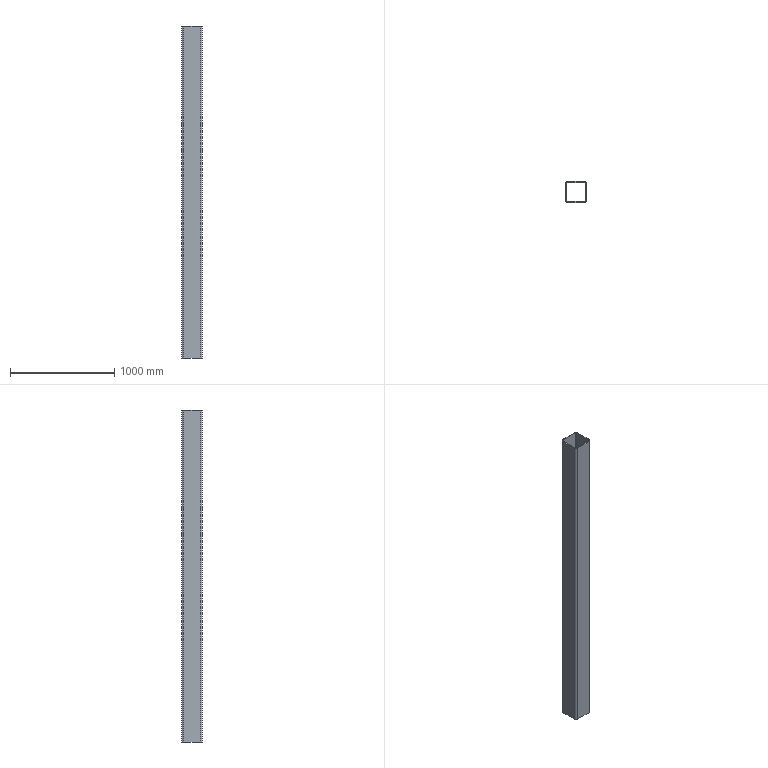Part | SolidWorks | features Extrusion 1 | 1 solid | 18 faces | box 200 x 200 x 3180 mm | volume 18839108 mm3 | plane 10 | cylinder 8 | commonest cylinder face diameters 24 x4 40 x4
STEP:
#1=CARTESIAN_POINT('',(-100.,-80.,3180.));
#2=VERTEX_POINT('',#1);
#3=CARTESIAN_POINT('',(-80.,-100.,3180.));
#4=VERTEX_POINT('',#3);
#5=CARTESIAN_POINT('',(-80.,-80.,3180.));
#6=DIRECTION('',(0.,0.,1.));
#7=DIRECTION('',(1.,0.,0.));
#8=AXIS2_PLACEMENT_3D('',#5,#6,#7);
#9=CIRCLE('',#8,20.);
#10=EDGE_CURVE('',#2,#4,#9,.T.);
#11=ORIENTED_EDGE('',*,*,#10,.T.);
#12=CARTESIAN_POINT('',(80.,-100.,3180.));
#13=VERTEX_POINT('',#12);
#14=CARTESIAN_POINT('',(-80.,-100.,3180.));
#15=DIRECTION('',(1.,0.,0.));
#16=VECTOR('',#15,1000.);
#17=LINE('',#14,#16);
#18=EDGE_CURVE('',#4,#13,#17,.T.);
#19=ORIENTED_EDGE('',*,*,#18,.T.);
#20=CARTESIAN_POINT('',(100.,-80.,3180.));
#21=VERTEX_POINT('',#20);
#22=CARTESIAN_POINT('',(80.,-80.,3180.));
#23=DIRECTION('',(0.,0.,1.));
#24=DIRECTION('',(1.,0.,0.));
#25=AXIS2_PLACEMENT_3D('',#22,#23,#24);
#26=CIRCLE('',#25,20.);
#27=EDGE_CURVE('',#13,#21,#26,.T.);
#28=ORIENTED_EDGE('',*,*,#27,.T.);
#29=CARTESIAN_POINT('',(100.,80.,3180.));
#30=VERTEX_POINT('',#29);
#31=CARTESIAN_POINT('',(100.,80.,3180.));
#32=DIRECTION('',(0.,1.,0.));
#33=VECTOR('',#32,1000.);
#34=LINE('',#31,#33);
#35=EDGE_CURVE('',#21,#30,#34,.T.);
#36=ORIENTED_EDGE('',*,*,#35,.T.);
#37=CARTESIAN_POINT('',(80.,100.,3180.));
#38=VERTEX_POINT('',#37);
#39=CARTESIAN_POINT('',(80.,80.,3180.));
#40=DIRECTION('',(0.,0.,1.));
#41=DIRECTION('',(-1.,0.,0.));
#42=AXIS2_PLACEMENT_3D('',#39,#40,#41);
#43=CIRCLE('',#42,20.);
#44=EDGE_CURVE('',#30,#38,#43,.T.);
#45=ORIENTED_EDGE('',*,*,#44,.T.);
#46=CARTESIAN_POINT('',(-80.,100.,3180.));
#47=VERTEX_POINT('',#46);
#48=CARTESIAN_POINT('',(-80.,100.,3180.));
#49=DIRECTION('',(-1.,0.,0.));
#50=VECTOR('',#49,1000.);
#51=LINE('',#48,#50);
#52=EDGE_CURVE('',#38,#47,#51,.T.);
#53=ORIENTED_EDGE('',*,*,#52,.T.);
#54=CARTESIAN_POINT('',(-100.,80.,3180.));
#55=VERTEX_POINT('',#54);
#56=CARTESIAN_POINT('',(-80.,80.,3180.));
#57=DIRECTION('',(0.,0.,1.));
#58=DIRECTION('',(1.,0.,0.));
#59=AXIS2_PLACEMENT_3D('',#56,#57,#58);
#60=CIRCLE('',#59,20.);
#61=EDGE_CURVE('',#47,#55,#60,.T.);
#62=ORIENTED_EDGE('',*,*,#61,.T.);
#63=CARTESIAN_POINT('',(-100.,80.,3180.));
#64=DIRECTION('',(0.,-1.,0.));
#65=VECTOR('',#64,1000.);
#66=LINE('',#63,#65);
#67=EDGE_CURVE('',#55,#2,#66,.T.);
#68=ORIENTED_EDGE('',*,*,#67,.T.);
#69=EDGE_LOOP('',(#11,#19,#28,#36,#45,#53,#62,#68));
#70=FACE_OUTER_BOUND('',#69,.T.);
#71=CARTESIAN_POINT('',(-92.,80.,3180.));
#72=VERTEX_POINT('',#71);
#73=CARTESIAN_POINT('',(-92.,-80.,3180.));
#74=VERTEX_POINT('',#73);
#75=CARTESIAN_POINT('',(-92.,80.,3180.));
#76=DIRECTION('',(0.,-1.,0.));
#77=VECTOR('',#76,1000.);
#78=LINE('',#75,#77);
#79=EDGE_CURVE('',#72,#74,#78,.T.);
#80=ORIENTED_EDGE('',*,*,#79,.F.);
#81=CARTESIAN_POINT('',(-80.,92.,3180.));
#82=VERTEX_POINT('',#81);
#83=CARTESIAN_POINT('',(-80.,80.,3180.));
#84=DIRECTION('',(0.,0.,1.));
#85=DIRECTION('',(1.,0.,0.));
#86=AXIS2_PLACEMENT_3D('',#83,#84,#85);
#87=CIRCLE('',#86,12.);
#88=EDGE_CURVE('',#82,#72,#87,.T.);
#89=ORIENTED_EDGE('',*,*,#88,.F.);
#90=CARTESIAN_POINT('',(80.,92.,3180.));
#91=VERTEX_POINT('',#90);
#92=CARTESIAN_POINT('',(-80.,92.,3180.));
#93=DIRECTION('',(-1.,0.,0.));
#94=VECTOR('',#93,1000.);
#95=LINE('',#92,#94);
#96=EDGE_CURVE('',#91,#82,#95,.T.);
#97=ORIENTED_EDGE('',*,*,#96,.F.);
#98=CARTESIAN_POINT('',(92.,80.,3180.));
#99=VERTEX_POINT('',#98);
#100=CARTESIAN_POINT('',(80.,80.,3180.));
#101=DIRECTION('',(0.,0.,1.));
#102=DIRECTION('',(-1.,0.,0.));
#103=AXIS2_PLACEMENT_3D('',#100,#101,#102);
#104=CIRCLE('',#103,12.);
#105=EDGE_CURVE('',#99,#91,#104,.T.);
#106=ORIENTED_EDGE('',*,*,#105,.F.);
#107=CARTESIAN_POINT('',(92.,-80.,3180.));
#108=VERTEX_POINT('',#107);
#109=CARTESIAN_POINT('',(92.,80.,3180.));
#110=DIRECTION('',(0.,1.,0.));
#111=VECTOR('',#110,1000.);
#112=LINE('',#109,#111);
#113=EDGE_CURVE('',#108,#99,#112,.T.);
#114=ORIENTED_EDGE('',*,*,#113,.F.);
#115=CARTESIAN_POINT('',(80.,-92.,3180.));
#116=VERTEX_POINT('',#115);
#117=CARTESIAN_POINT('',(80.,-80.,3180.));
#118=DIRECTION('',(0.,0.,1.));
#119=DIRECTION('',(1.,0.,0.));
#120=AXIS2_PLACEMENT_3D('',#117,#118,#119);
#121=CIRCLE('',#120,12.);
#122=EDGE_CURVE('',#116,#108,#121,.T.);
#123=ORIENTED_EDGE('',*,*,#122,.F.);
#124=CARTESIAN_POINT('',(-80.,-92.,3180.));
#125=VERTEX_POINT('',#124);
#126=CARTESIAN_POINT('',(-80.,-92.,3180.));
#127=DIRECTION('',(1.,0.,0.));
#128=VECTOR('',#127,1000.);
#129=LINE('',#126,#128);
#130=EDGE_CURVE('',#125,#116,#129,.T.);
#131=ORIENTED_EDGE('',*,*,#130,.F.);
#132=CARTESIAN_POINT('',(-80.,-80.,3180.));
#133=DIRECTION('',(0.,0.,1.));
#134=DIRECTION('',(1.,0.,0.));
#135=AXIS2_PLACEMENT_3D('',#132,#133,#134);
#136=CIRCLE('',#135,12.);
#137=EDGE_CURVE('',#74,#125,#136,.T.);
#138=ORIENTED_EDGE('',*,*,#137,.F.);
#139=EDGE_LOOP('',(#80,#89,#97,#106,#114,#123,#131,#138));
#140=FACE_BOUND('',#139,.T.);
#141=CARTESIAN_POINT('',(-80.,-80.,3180.));
#142=DIRECTION('',(0.,0.,1.));
#143=DIRECTION('',(1.,0.,0.));
#144=AXIS2_PLACEMENT_3D('',#141,#142,#143);
#145=PLANE('',#144);
#146=ADVANCED_FACE('',(#70,#140),#145,.T.);
#147=CARTESIAN_POINT('',(-100.,-80.,0.));
#148=VERTEX_POINT('',#147);
#149=CARTESIAN_POINT('',(-80.,-100.,0.));
#150=VERTEX_POINT('',#149);
#151=CARTESIAN_POINT('',(-80.,-80.,0.));
#152=DIRECTION('',(0.,0.,1.));
#153=DIRECTION('',(1.,0.,0.));
#154=AXIS2_PLACEMENT_3D('',#151,#152,#153);
#155=CIRCLE('',#154,20.);
#156=EDGE_CURVE('',#148,#150,#155,.T.);
#157=ORIENTED_EDGE('',*,*,#156,.F.);
#158=CARTESIAN_POINT('',(-100.,80.,0.));
#159=VERTEX_POINT('',#158);
#160=CARTESIAN_POINT('',(-100.,80.,0.));
#161=DIRECTION('',(0.,-1.,0.));
#162=VECTOR('',#161,1000.);
#163=LINE('',#160,#162);
#164=EDGE_CURVE('',#159,#148,#163,.T.);
#165=ORIENTED_EDGE('',*,*,#164,.F.);
#166=CARTESIAN_POINT('',(-80.,100.,0.));
#167=VERTEX_POINT('',#166);
#168=CARTESIAN_POINT('',(-80.,80.,0.));
#169=DIRECTION('',(0.,0.,1.));
#170=DIRECTION('',(1.,0.,0.));
#171=AXIS2_PLACEMENT_3D('',#168,#169,#170);
#172=CIRCLE('',#171,20.);
#173=EDGE_CURVE('',#167,#159,#172,.T.);
#174=ORIENTED_EDGE('',*,*,#173,.F.);
#175=CARTESIAN_POINT('',(80.,100.,0.));
#176=VERTEX_POINT('',#175);
#177=CARTESIAN_POINT('',(-80.,100.,0.));
#178=DIRECTION('',(-1.,0.,0.));
#179=VECTOR('',#178,1000.);
#180=LINE('',#177,#179);
#181=EDGE_CURVE('',#176,#167,#180,.T.);
#182=ORIENTED_EDGE('',*,*,#181,.F.);
#183=CARTESIAN_POINT('',(100.,80.,0.));
#184=VERTEX_POINT('',#183);
#185=CARTESIAN_POINT('',(80.,80.,0.));
#186=DIRECTION('',(0.,0.,1.));
#187=DIRECTION('',(-1.,0.,0.));
#188=AXIS2_PLACEMENT_3D('',#185,#186,#187);
#189=CIRCLE('',#188,20.);
#190=EDGE_CURVE('',#184,#176,#189,.T.);
#191=ORIENTED_EDGE('',*,*,#190,.F.);
#192=CARTESIAN_POINT('',(100.,-80.,0.));
#193=VERTEX_POINT('',#192);
#194=CARTESIAN_POINT('',(100.,80.,0.));
#195=DIRECTION('',(0.,1.,0.));
#196=VECTOR('',#195,1000.);
#197=LINE('',#194,#196);
#198=EDGE_CURVE('',#193,#184,#197,.T.);
#199=ORIENTED_EDGE('',*,*,#198,.F.);
#200=CARTESIAN_POINT('',(80.,-100.,0.));
#201=VERTEX_POINT('',#200);
#202=CARTESIAN_POINT('',(80.,-80.,0.));
#203=DIRECTION('',(0.,0.,1.));
#204=DIRECTION('',(1.,0.,0.));
#205=AXIS2_PLACEMENT_3D('',#202,#203,#204);
#206=CIRCLE('',#205,20.);
#207=EDGE_CURVE('',#201,#193,#206,.T.);
#208=ORIENTED_EDGE('',*,*,#207,.F.);
#209=CARTESIAN_POINT('',(-80.,-100.,0.));
#210=DIRECTION('',(1.,0.,0.));
#211=VECTOR('',#210,1000.);
#212=LINE('',#209,#211);
#213=EDGE_CURVE('',#150,#201,#212,.T.);
#214=ORIENTED_EDGE('',*,*,#213,.F.);
#215=EDGE_LOOP('',(#157,#165,#174,#182,#191,#199,#208,#214));
#216=FACE_OUTER_BOUND('',#215,.T.);
#217=CARTESIAN_POINT('',(-80.,92.,0.));
#218=VERTEX_POINT('',#217);
#219=CARTESIAN_POINT('',(-92.,80.,0.));
#220=VERTEX_POINT('',#219);
#221=CARTESIAN_POINT('',(-80.,80.,0.));
#222=DIRECTION('',(0.,0.,1.));
#223=DIRECTION('',(1.,0.,0.));
#224=AXIS2_PLACEMENT_3D('',#221,#222,#223);
#225=CIRCLE('',#224,12.);
#226=EDGE_CURVE('',#218,#220,#225,.T.);
#227=ORIENTED_EDGE('',*,*,#226,.T.);
#228=CARTESIAN_POINT('',(-92.,-80.,0.));
#229=VERTEX_POINT('',#228);
#230=CARTESIAN_POINT('',(-92.,80.,0.));
#231=DIRECTION('',(0.,-1.,0.));
#232=VECTOR('',#231,1000.);
#233=LINE('',#230,#232);
#234=EDGE_CURVE('',#220,#229,#233,.T.);
#235=ORIENTED_EDGE('',*,*,#234,.T.);
#236=CARTESIAN_POINT('',(-80.,-92.,0.));
#237=VERTEX_POINT('',#236);
#238=CARTESIAN_POINT('',(-80.,-80.,0.));
#239=DIRECTION('',(0.,0.,1.));
#240=DIRECTION('',(1.,0.,0.));
#241=AXIS2_PLACEMENT_3D('',#238,#239,#240);
#242=CIRCLE('',#241,12.);
#243=EDGE_CURVE('',#229,#237,#242,.T.);
#244=ORIENTED_EDGE('',*,*,#243,.T.);
#245=CARTESIAN_POINT('',(80.,-92.,0.));
#246=VERTEX_POINT('',#245);
#247=CARTESIAN_POINT('',(-80.,-92.,0.));
#248=DIRECTION('',(1.,0.,0.));
#249=VECTOR('',#248,1000.);
#250=LINE('',#247,#249);
#251=EDGE_CURVE('',#237,#246,#250,.T.);
#252=ORIENTED_EDGE('',*,*,#251,.T.);
#253=CARTESIAN_POINT('',(92.,-80.,0.));
#254=VERTEX_POINT('',#253);
#255=CARTESIAN_POINT('',(80.,-80.,0.));
#256=DIRECTION('',(0.,0.,1.));
#257=DIRECTION('',(1.,0.,0.));
#258=AXIS2_PLACEMENT_3D('',#255,#256,#257);
#259=CIRCLE('',#258,12.);
#260=EDGE_CURVE('',#246,#254,#259,.T.);
#261=ORIENTED_EDGE('',*,*,#260,.T.);
#262=CARTESIAN_POINT('',(92.,80.,0.));
#263=VERTEX_POINT('',#262);
#264=CARTESIAN_POINT('',(92.,80.,0.));
#265=DIRECTION('',(0.,1.,0.));
#266=VECTOR('',#265,1000.);
#267=LINE('',#264,#266);
#268=EDGE_CURVE('',#254,#263,#267,.T.);
#269=ORIENTED_EDGE('',*,*,#268,.T.);
#270=CARTESIAN_POINT('',(80.,92.,0.));
#271=VERTEX_POINT('',#270);
#272=CARTESIAN_POINT('',(80.,80.,0.));
#273=DIRECTION('',(0.,0.,1.));
#274=DIRECTION('',(-1.,0.,0.));
#275=AXIS2_PLACEMENT_3D('',#272,#273,#274);
#276=CIRCLE('',#275,12.);
#277=EDGE_CURVE('',#263,#271,#276,.T.);
#278=ORIENTED_EDGE('',*,*,#277,.T.);
#279=CARTESIAN_POINT('',(-80.,92.,0.));
#280=DIRECTION('',(-1.,0.,0.));
#281=VECTOR('',#280,1000.);
#282=LINE('',#279,#281);
#283=EDGE_CURVE('',#271,#218,#282,.T.);
#284=ORIENTED_EDGE('',*,*,#283,.T.);
#285=EDGE_LOOP('',(#227,#235,#244,#252,#261,#269,#278,#284));
#286=FACE_BOUND('',#285,.T.);
#287=CARTESIAN_POINT('',(-80.,-80.,0.));
#288=DIRECTION('',(0.,0.,1.));
#289=DIRECTION('',(1.,0.,0.));
#290=AXIS2_PLACEMENT_3D('',#287,#288,#289);
#291=PLANE('',#290);
#292=ADVANCED_FACE('',(#216,#286),#291,.F.);
#293=ORIENTED_EDGE('',*,*,#156,.T.);
#294=CARTESIAN_POINT('',(-80.,-100.,3180.));
#295=DIRECTION('',(0.,0.,-1.));
#296=VECTOR('',#295,1000.);
#297=LINE('',#294,#296);
#298=EDGE_CURVE('',#4,#150,#297,.T.);
#299=ORIENTED_EDGE('',*,*,#298,.F.);
#300=ORIENTED_EDGE('',*,*,#10,.F.);
#301=CARTESIAN_POINT('',(-100.,-80.,3180.));
#302=DIRECTION('',(0.,0.,-1.));
#303=VECTOR('',#302,1000.);
#304=LINE('',#301,#303);
#305=EDGE_CURVE('',#2,#148,#304,.T.);
#306=ORIENTED_EDGE('',*,*,#305,.T.);
#307=EDGE_LOOP('',(#293,#299,#300,#306));
#308=FACE_OUTER_BOUND('',#307,.T.);
#309=CARTESIAN_POINT('',(-80.,-80.,3180.));
#310=DIRECTION('',(0.,0.,-1.));
#311=DIRECTION('',(-1.,0.,0.));
#312=AXIS2_PLACEMENT_3D('',#309,#310,#311);
#313=CYLINDRICAL_SURFACE('',#312,20.);
#314=ADVANCED_FACE('',(#308),#313,.T.);
#315=ORIENTED_EDGE('',*,*,#213,.T.);
#316=CARTESIAN_POINT('',(80.,-100.,3180.));
#317=DIRECTION('',(0.,0.,-1.));
#318=VECTOR('',#317,1000.);
#319=LINE('',#316,#318);
#320=EDGE_CURVE('',#13,#201,#319,.T.);
#321=ORIENTED_EDGE('',*,*,#320,.F.);
#322=ORIENTED_EDGE('',*,*,#18,.F.);
#323=ORIENTED_EDGE('',*,*,#298,.T.);
#324=EDGE_LOOP('',(#315,#321,#322,#323));
#325=FACE_OUTER_BOUND('',#324,.T.);
#326=CARTESIAN_POINT('',(-80.,-100.,3180.));
#327=DIRECTION('',(0.,1.,0.));
#328=DIRECTION('',(0.,0.,1.));
#329=AXIS2_PLACEMENT_3D('',#326,#327,#328);
#330=PLANE('',#329);
#331=ADVANCED_FACE('',(#325),#330,.F.);
#332=ORIENTED_EDGE('',*,*,#207,.T.);
#333=CARTESIAN_POINT('',(100.,-80.,3180.));
#334=DIRECTION('',(0.,0.,-1.));
#335=VECTOR('',#334,1000.);
#336=LINE('',#333,#335);
#337=EDGE_CURVE('',#21,#193,#336,.T.);
#338=ORIENTED_EDGE('',*,*,#337,.F.);
#339=ORIENTED_EDGE('',*,*,#27,.F.);
#340=ORIENTED_EDGE('',*,*,#320,.T.);
#341=EDGE_LOOP('',(#332,#338,#339,#340));
#342=FACE_OUTER_BOUND('',#341,.T.);
#343=CARTESIAN_POINT('',(80.,-80.,3180.));
#344=DIRECTION('',(0.,0.,-1.));
#345=DIRECTION('',(-1.,0.,0.));
#346=AXIS2_PLACEMENT_3D('',#343,#344,#345);
#347=CYLINDRICAL_SURFACE('',#346,20.);
#348=ADVANCED_FACE('',(#342),#347,.T.);
#349=ORIENTED_EDGE('',*,*,#198,.T.);
#350=CARTESIAN_POINT('',(100.,80.,3180.));
#351=DIRECTION('',(0.,0.,-1.));
#352=VECTOR('',#351,1000.);
#353=LINE('',#350,#352);
#354=EDGE_CURVE('',#30,#184,#353,.T.);
#355=ORIENTED_EDGE('',*,*,#354,.F.);
#356=ORIENTED_EDGE('',*,*,#35,.F.);
#357=ORIENTED_EDGE('',*,*,#337,.T.);
#358=EDGE_LOOP('',(#349,#355,#356,#357));
#359=FACE_OUTER_BOUND('',#358,.T.);
#360=CARTESIAN_POINT('',(100.,80.,3180.));
#361=DIRECTION('',(-1.,0.,0.));
#362=DIRECTION('',(0.,-1.,0.));
#363=AXIS2_PLACEMENT_3D('',#360,#361,#362);
#364=PLANE('',#363);
#365=ADVANCED_FACE('',(#359),#364,.F.);
#366=ORIENTED_EDGE('',*,*,#190,.T.);
#367=CARTESIAN_POINT('',(80.,100.,3180.));
#368=DIRECTION('',(0.,0.,-1.));
#369=VECTOR('',#368,1000.);
#370=LINE('',#367,#369);
#371=EDGE_CURVE('',#38,#176,#370,.T.);
#372=ORIENTED_EDGE('',*,*,#371,.F.);
#373=ORIENTED_EDGE('',*,*,#44,.F.);
#374=ORIENTED_EDGE('',*,*,#354,.T.);
#375=EDGE_LOOP('',(#366,#372,#373,#374));
#376=FACE_OUTER_BOUND('',#375,.T.);
#377=CARTESIAN_POINT('',(80.,80.,3180.));
#378=DIRECTION('',(0.,0.,-1.));
#379=DIRECTION('',(-1.,0.,0.));
#380=AXIS2_PLACEMENT_3D('',#377,#378,#379);
#381=CYLINDRICAL_SURFACE('',#380,20.);
#382=ADVANCED_FACE('',(#376),#381,.T.);
#383=ORIENTED_EDGE('',*,*,#181,.T.);
#384=CARTESIAN_POINT('',(-80.,100.,3180.));
#385=DIRECTION('',(0.,0.,-1.));
#386=VECTOR('',#385,1000.);
#387=LINE('',#384,#386);
#388=EDGE_CURVE('',#47,#167,#387,.T.);
#389=ORIENTED_EDGE('',*,*,#388,.F.);
#390=ORIENTED_EDGE('',*,*,#52,.F.);
#391=ORIENTED_EDGE('',*,*,#371,.T.);
#392=EDGE_LOOP('',(#383,#389,#390,#391));
#393=FACE_OUTER_BOUND('',#392,.T.);
#394=CARTESIAN_POINT('',(-80.,100.,3180.));
#395=DIRECTION('',(0.,-1.,0.));
#396=DIRECTION('',(0.,0.,-1.));
#397=AXIS2_PLACEMENT_3D('',#394,#395,#396);
#398=PLANE('',#397);
#399=ADVANCED_FACE('',(#393),#398,.F.);
#400=ORIENTED_EDGE('',*,*,#173,.T.);
#401=CARTESIAN_POINT('',(-100.,80.,3180.));
#402=DIRECTION('',(0.,0.,-1.));
#403=VECTOR('',#402,1000.);
#404=LINE('',#401,#403);
#405=EDGE_CURVE('',#55,#159,#404,.T.);
#406=ORIENTED_EDGE('',*,*,#405,.F.);
#407=ORIENTED_EDGE('',*,*,#61,.F.);
#408=ORIENTED_EDGE('',*,*,#388,.T.);
#409=EDGE_LOOP('',(#400,#406,#407,#408));
#410=FACE_OUTER_BOUND('',#409,.T.);
#411=CARTESIAN_POINT('',(-80.,80.,3180.));
#412=DIRECTION('',(0.,0.,-1.));
#413=DIRECTION('',(-1.,0.,0.));
#414=AXIS2_PLACEMENT_3D('',#411,#412,#413);
#415=CYLINDRICAL_SURFACE('',#414,20.);
#416=ADVANCED_FACE('',(#410),#415,.T.);
#417=ORIENTED_EDGE('',*,*,#164,.T.);
#418=ORIENTED_EDGE('',*,*,#305,.F.);
#419=ORIENTED_EDGE('',*,*,#67,.F.);
#420=ORIENTED_EDGE('',*,*,#405,.T.);
#421=EDGE_LOOP('',(#417,#418,#419,#420));
#422=FACE_OUTER_BOUND('',#421,.T.);
#423=CARTESIAN_POINT('',(-100.,80.,3180.));
#424=DIRECTION('',(1.,0.,0.));
#425=DIRECTION('',(0.,1.,0.));
#426=AXIS2_PLACEMENT_3D('',#423,#424,#425);
#427=PLANE('',#426);
#428=ADVANCED_FACE('',(#422),#427,.F.);
#429=ORIENTED_EDGE('',*,*,#226,.F.);
#430=CARTESIAN_POINT('',(-80.,92.,3180.));
#431=DIRECTION('',(0.,0.,-1.));
#432=VECTOR('',#431,1000.);
#433=LINE('',#430,#432);
#434=EDGE_CURVE('',#82,#218,#433,.T.);
#435=ORIENTED_EDGE('',*,*,#434,.F.);
#436=ORIENTED_EDGE('',*,*,#88,.T.);
#437=CARTESIAN_POINT('',(-92.,80.,3180.));
#438=DIRECTION('',(0.,0.,-1.));
#439=VECTOR('',#438,1000.);
#440=LINE('',#437,#439);
#441=EDGE_CURVE('',#72,#220,#440,.T.);
#442=ORIENTED_EDGE('',*,*,#441,.T.);
#443=EDGE_LOOP('',(#429,#435,#436,#442));
#444=FACE_OUTER_BOUND('',#443,.T.);
#445=CARTESIAN_POINT('',(-80.,80.,3180.));
#446=DIRECTION('',(0.,0.,-1.));
#447=DIRECTION('',(-1.,0.,0.));
#448=AXIS2_PLACEMENT_3D('',#445,#446,#447);
#449=CYLINDRICAL_SURFACE('',#448,12.);
#450=ADVANCED_FACE('',(#444),#449,.F.);
#451=ORIENTED_EDGE('',*,*,#234,.F.);
#452=ORIENTED_EDGE('',*,*,#441,.F.);
#453=ORIENTED_EDGE('',*,*,#79,.T.);
#454=CARTESIAN_POINT('',(-92.,-80.,3180.));
#455=DIRECTION('',(0.,0.,-1.));
#456=VECTOR('',#455,1000.);
#457=LINE('',#454,#456);
#458=EDGE_CURVE('',#74,#229,#457,.T.);
#459=ORIENTED_EDGE('',*,*,#458,.T.);
#460=EDGE_LOOP('',(#451,#452,#453,#459));
#461=FACE_OUTER_BOUND('',#460,.T.);
#462=CARTESIAN_POINT('',(-92.,80.,3180.));
#463=DIRECTION('',(1.,0.,0.));
#464=DIRECTION('',(0.,0.,-1.));
#465=AXIS2_PLACEMENT_3D('',#462,#463,#464);
#466=PLANE('',#465);
#467=ADVANCED_FACE('',(#461),#466,.T.);
#468=ORIENTED_EDGE('',*,*,#243,.F.);
#469=ORIENTED_EDGE('',*,*,#458,.F.);
#470=ORIENTED_EDGE('',*,*,#137,.T.);
#471=CARTESIAN_POINT('',(-80.,-92.,3180.));
#472=DIRECTION('',(0.,0.,-1.));
#473=VECTOR('',#472,1000.);
#474=LINE('',#471,#473);
#475=EDGE_CURVE('',#125,#237,#474,.T.);
#476=ORIENTED_EDGE('',*,*,#475,.T.);
#477=EDGE_LOOP('',(#468,#469,#470,#476));
#478=FACE_OUTER_BOUND('',#477,.T.);
#479=CARTESIAN_POINT('',(-80.,-80.,3180.));
#480=DIRECTION('',(0.,0.,-1.));
#481=DIRECTION('',(-1.,0.,0.));
#482=AXIS2_PLACEMENT_3D('',#479,#480,#481);
#483=CYLINDRICAL_SURFACE('',#482,12.);
#484=ADVANCED_FACE('',(#478),#483,.F.);
#485=ORIENTED_EDGE('',*,*,#251,.F.);
#486=ORIENTED_EDGE('',*,*,#475,.F.);
#487=ORIENTED_EDGE('',*,*,#130,.T.);
#488=CARTESIAN_POINT('',(80.,-92.,3180.));
#489=DIRECTION('',(0.,0.,-1.));
#490=VECTOR('',#489,1000.);
#491=LINE('',#488,#490);
#492=EDGE_CURVE('',#116,#246,#491,.T.);
#493=ORIENTED_EDGE('',*,*,#492,.T.);
#494=EDGE_LOOP('',(#485,#486,#487,#493));
#495=FACE_OUTER_BOUND('',#494,.T.);
#496=CARTESIAN_POINT('',(-80.,-92.,3180.));
#497=DIRECTION('',(0.,1.,0.));
#498=DIRECTION('',(0.,0.,1.));
#499=AXIS2_PLACEMENT_3D('',#496,#497,#498);
#500=PLANE('',#499);
#501=ADVANCED_FACE('',(#495),#500,.T.);
#502=ORIENTED_EDGE('',*,*,#260,.F.);
#503=ORIENTED_EDGE('',*,*,#492,.F.);
#504=ORIENTED_EDGE('',*,*,#122,.T.);
#505=CARTESIAN_POINT('',(92.,-80.,3180.));
#506=DIRECTION('',(0.,0.,-1.));
#507=VECTOR('',#506,1000.);
#508=LINE('',#505,#507);
#509=EDGE_CURVE('',#108,#254,#508,.T.);
#510=ORIENTED_EDGE('',*,*,#509,.T.);
#511=EDGE_LOOP('',(#502,#503,#504,#510));
#512=FACE_OUTER_BOUND('',#511,.T.);
#513=CARTESIAN_POINT('',(80.,-80.,3180.));
#514=DIRECTION('',(0.,0.,-1.));
#515=DIRECTION('',(-1.,0.,0.));
#516=AXIS2_PLACEMENT_3D('',#513,#514,#515);
#517=CYLINDRICAL_SURFACE('',#516,12.);
#518=ADVANCED_FACE('',(#512),#517,.F.);
#519=ORIENTED_EDGE('',*,*,#268,.F.);
#520=ORIENTED_EDGE('',*,*,#509,.F.);
#521=ORIENTED_EDGE('',*,*,#113,.T.);
#522=CARTESIAN_POINT('',(92.,80.,3180.));
#523=DIRECTION('',(0.,0.,-1.));
#524=VECTOR('',#523,1000.);
#525=LINE('',#522,#524);
#526=EDGE_CURVE('',#99,#263,#525,.T.);
#527=ORIENTED_EDGE('',*,*,#526,.T.);
#528=EDGE_LOOP('',(#519,#520,#521,#527));
#529=FACE_OUTER_BOUND('',#528,.T.);
#530=CARTESIAN_POINT('',(92.,80.,3180.));
#531=DIRECTION('',(-1.,0.,0.));
#532=DIRECTION('',(0.,-1.,0.));
#533=AXIS2_PLACEMENT_3D('',#530,#531,#532);
#534=PLANE('',#533);
#535=ADVANCED_FACE('',(#529),#534,.T.);
#536=ORIENTED_EDGE('',*,*,#277,.F.);
#537=ORIENTED_EDGE('',*,*,#526,.F.);
#538=ORIENTED_EDGE('',*,*,#105,.T.);
#539=CARTESIAN_POINT('',(80.,92.,3180.));
#540=DIRECTION('',(0.,0.,-1.));
#541=VECTOR('',#540,1000.);
#542=LINE('',#539,#541);
#543=EDGE_CURVE('',#91,#271,#542,.T.);
#544=ORIENTED_EDGE('',*,*,#543,.T.);
#545=EDGE_LOOP('',(#536,#537,#538,#544));
#546=FACE_OUTER_BOUND('',#545,.T.);
#547=CARTESIAN_POINT('',(80.,80.,3180.));
#548=DIRECTION('',(0.,0.,-1.));
#549=DIRECTION('',(-1.,0.,0.));
#550=AXIS2_PLACEMENT_3D('',#547,#548,#549);
#551=CYLINDRICAL_SURFACE('',#550,12.);
#552=ADVANCED_FACE('',(#546),#551,.F.);
#553=ORIENTED_EDGE('',*,*,#283,.F.);
#554=ORIENTED_EDGE('',*,*,#543,.F.);
#555=ORIENTED_EDGE('',*,*,#96,.T.);
#556=ORIENTED_EDGE('',*,*,#434,.T.);
#557=EDGE_LOOP('',(#553,#554,#555,#556));
#558=FACE_OUTER_BOUND('',#557,.T.);
#559=CARTESIAN_POINT('',(-80.,92.,3180.));
#560=DIRECTION('',(0.,-1.,0.));
#561=DIRECTION('',(0.,0.,-1.));
#562=AXIS2_PLACEMENT_3D('',#559,#560,#561);
#563=PLANE('',#562);
#564=ADVANCED_FACE('',(#558),#563,.T.);
#565=CLOSED_SHELL('',(#146,#292,#314,#331,#348,#365,#382,#399,#416,#428,#450,#467,#484,#501,#518,#535,#552,#564));
#566=MANIFOLD_SOLID_BREP('',#565);
#567=CARTESIAN_POINT('',(0.,0.,0.));
#568=DIRECTION('',(0.,0.,1.));
#569=DIRECTION('',(1.,0.,0.));
#570=AXIS2_PLACEMENT_3D('',#567,#568,#569);
#571=(LENGTH_UNIT()NAMED_UNIT(*)SI_UNIT(.MILLI.,.METRE.));
#572=UNCERTAINTY_MEASURE_WITH_UNIT(LENGTH_MEASURE(0.00001),#571,'','');
#573=(NAMED_UNIT(*)PLANE_ANGLE_UNIT()SI_UNIT($,.RADIAN.));
#574=(NAMED_UNIT(*)SI_UNIT($,.STERADIAN.)SOLID_ANGLE_UNIT());
#575=(GEOMETRIC_REPRESENTATION_CONTEXT(3)GLOBAL_UNCERTAINTY_ASSIGNED_CONTEXT((#572))GLOBAL_UNIT_ASSIGNED_CONTEXT((#571,#573,#574))REPRESENTATION_CONTEXT('',''));
#576=ADVANCED_BREP_SHAPE_REPRESENTATION('',(#566,#570),#575);